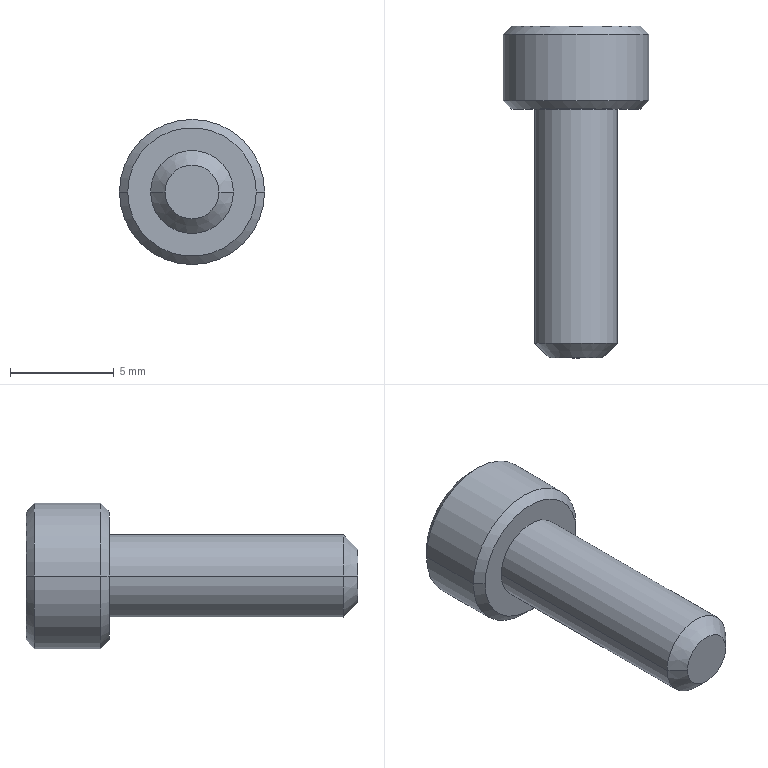Part | STEP file | BB62-M4-12L-1 | 1 solid | 27 faces | box 7 x 16 x 7 mm | volume 280.182 mm3 | plane 15 | cone 8 | cylinder 4 | commonest cylinder face diameters 4 x2 7 x2
STEP:
#1=CARTESIAN_POINT('',(0.,1.007,0.));
#2=VERTEX_POINT('',#1);
#3=CARTESIAN_POINT('',(1.72,2.,0.));
#4=VERTEX_POINT('',#3);
#5=CARTESIAN_POINT('',(0.,1.007,0.));
#6=DIRECTION('',(0.866,0.5,0.));
#7=VECTOR('',#6,1000.);
#8=LINE('',#5,#7);
#9=EDGE_CURVE('',#2,#4,#8,.T.);
#10=ORIENTED_EDGE('',*,*,#9,.F.);
#11=CARTESIAN_POINT('',(-1.72,2.,0.));
#12=VERTEX_POINT('',#11);
#13=CARTESIAN_POINT('',(0.,1.007,0.));
#14=DIRECTION('',(-0.866,0.5,0.));
#15=VECTOR('',#14,1000.);
#16=LINE('',#13,#15);
#17=EDGE_CURVE('',#2,#12,#16,.T.);
#18=ORIENTED_EDGE('',*,*,#17,.T.);
#19=CARTESIAN_POINT('',(-1.49,2.,0.86));
#20=VERTEX_POINT('',#19);
#21=CARTESIAN_POINT('',(0.,2.,0.));
#22=DIRECTION('',(0.,-1.,0.));
#23=DIRECTION('',(-1.,0.,0.));
#24=AXIS2_PLACEMENT_3D('',#21,#22,#23);
#25=CIRCLE('',#24,1.72);
#26=EDGE_CURVE('',#20,#12,#25,.T.);
#27=ORIENTED_EDGE('',*,*,#26,.F.);
#28=CARTESIAN_POINT('',(0.,2.,1.72));
#29=VERTEX_POINT('',#28);
#30=CARTESIAN_POINT('',(0.,2.,0.));
#31=DIRECTION('',(0.,-1.,0.));
#32=DIRECTION('',(-1.,0.,0.));
#33=AXIS2_PLACEMENT_3D('',#30,#31,#32);
#34=CIRCLE('',#33,1.72);
#35=EDGE_CURVE('',#29,#20,#34,.T.);
#36=ORIENTED_EDGE('',*,*,#35,.F.);
#37=CARTESIAN_POINT('',(1.49,2.,0.86));
#38=VERTEX_POINT('',#37);
#39=CARTESIAN_POINT('',(0.,2.,0.));
#40=DIRECTION('',(0.,-1.,0.));
#41=DIRECTION('',(-1.,0.,0.));
#42=AXIS2_PLACEMENT_3D('',#39,#40,#41);
#43=CIRCLE('',#42,1.72);
#44=EDGE_CURVE('',#38,#29,#43,.T.);
#45=ORIENTED_EDGE('',*,*,#44,.F.);
#46=CARTESIAN_POINT('',(0.,2.,0.));
#47=DIRECTION('',(0.,-1.,0.));
#48=DIRECTION('',(-1.,0.,0.));
#49=AXIS2_PLACEMENT_3D('',#46,#47,#48);
#50=CIRCLE('',#49,1.72);
#51=EDGE_CURVE('',#4,#38,#50,.T.);
#52=ORIENTED_EDGE('',*,*,#51,.F.);
#53=EDGE_LOOP('',(#10,#18,#27,#36,#45,#52));
#54=FACE_OUTER_BOUND('',#53,.T.);
#55=CARTESIAN_POINT('',(0.,1001.007,0.));
#56=DIRECTION('',(0.,1.,0.));
#57=DIRECTION('',(1.,0.,0.));
#58=AXIS2_PLACEMENT_3D('',#55,#56,#57);
#59=CONICAL_SURFACE('',#58,1732.051,1.047);
#60=ADVANCED_FACE('',(#54),#59,.F.);
#61=CARTESIAN_POINT('',(1.3,-12.,0.));
#62=VERTEX_POINT('',#61);
#63=CARTESIAN_POINT('',(-1.3,-12.,0.));
#64=VERTEX_POINT('',#63);
#65=CARTESIAN_POINT('',(0.,-12.,0.));
#66=DIRECTION('',(0.,1.,0.));
#67=DIRECTION('',(1.,0.,0.));
#68=AXIS2_PLACEMENT_3D('',#65,#66,#67);
#69=CIRCLE('',#68,1.3);
#70=EDGE_CURVE('',#62,#64,#69,.T.);
#71=ORIENTED_EDGE('',*,*,#70,.T.);
#72=CARTESIAN_POINT('',(-2.,-11.3,0.));
#73=VERTEX_POINT('',#72);
#74=CARTESIAN_POINT('',(-1.3,-12.,0.));
#75=DIRECTION('',(-0.7071,0.7071,0.));
#76=VECTOR('',#75,1000.);
#77=LINE('',#74,#76);
#78=EDGE_CURVE('',#64,#73,#77,.T.);
#79=ORIENTED_EDGE('',*,*,#78,.T.);
#80=CARTESIAN_POINT('',(2.,-11.3,0.));
#81=VERTEX_POINT('',#80);
#82=CARTESIAN_POINT('',(0.,-11.3,0.));
#83=DIRECTION('',(0.,-1.,0.));
#84=DIRECTION('',(-1.,0.,0.));
#85=AXIS2_PLACEMENT_3D('',#82,#83,#84);
#86=CIRCLE('',#85,2.);
#87=EDGE_CURVE('',#73,#81,#86,.T.);
#88=ORIENTED_EDGE('',*,*,#87,.T.);
#89=CARTESIAN_POINT('',(1.3,-12.,0.));
#90=DIRECTION('',(0.7071,0.7071,0.));
#91=VECTOR('',#90,1000.);
#92=LINE('',#89,#91);
#93=EDGE_CURVE('',#62,#81,#92,.T.);
#94=ORIENTED_EDGE('',*,*,#93,.F.);
#95=EDGE_LOOP('',(#71,#79,#88,#94));
#96=FACE_OUTER_BOUND('',#95,.T.);
#97=CARTESIAN_POINT('',(0.,-12.,0.));
#98=DIRECTION('',(0.,1.,0.));
#99=DIRECTION('',(1.,0.,0.));
#100=AXIS2_PLACEMENT_3D('',#97,#98,#99);
#101=CONICAL_SURFACE('',#100,1.3,0.7854);
#102=ADVANCED_FACE('',(#96),#101,.T.);
#103=ORIENTED_EDGE('',*,*,#87,.F.);
#104=CARTESIAN_POINT('',(-2.,0.,0.));
#105=VERTEX_POINT('',#104);
#106=CARTESIAN_POINT('',(-2.,-11.3,0.));
#107=DIRECTION('',(0.,1.,0.));
#108=VECTOR('',#107,1000.);
#109=LINE('',#106,#108);
#110=EDGE_CURVE('',#73,#105,#109,.T.);
#111=ORIENTED_EDGE('',*,*,#110,.T.);
#112=CARTESIAN_POINT('',(2.,0.,0.));
#113=VERTEX_POINT('',#112);
#114=CARTESIAN_POINT('',(0.,0.,0.));
#115=DIRECTION('',(0.,-1.,0.));
#116=DIRECTION('',(-1.,0.,0.));
#117=AXIS2_PLACEMENT_3D('',#114,#115,#116);
#118=CIRCLE('',#117,2.);
#119=EDGE_CURVE('',#105,#113,#118,.T.);
#120=ORIENTED_EDGE('',*,*,#119,.T.);
#121=CARTESIAN_POINT('',(2.,-11.3,0.));
#122=DIRECTION('',(0.,1.,0.));
#123=VECTOR('',#122,1000.);
#124=LINE('',#121,#123);
#125=EDGE_CURVE('',#81,#113,#124,.T.);
#126=ORIENTED_EDGE('',*,*,#125,.F.);
#127=EDGE_LOOP('',(#103,#111,#120,#126));
#128=FACE_OUTER_BOUND('',#127,.T.);
#129=CARTESIAN_POINT('',(0.,-11.3,0.));
#130=DIRECTION('',(0.,1.,0.));
#131=DIRECTION('',(1.,0.,0.));
#132=AXIS2_PLACEMENT_3D('',#129,#130,#131);
#133=CYLINDRICAL_SURFACE('',#132,2.);
#134=ADVANCED_FACE('',(#128),#133,.T.);
#135=CARTESIAN_POINT('',(-3.1,4.,0.));
#136=VERTEX_POINT('',#135);
#137=CARTESIAN_POINT('',(3.1,4.,0.));
#138=VERTEX_POINT('',#137);
#139=CARTESIAN_POINT('',(0.,4.,0.));
#140=DIRECTION('',(0.,-1.,0.));
#141=DIRECTION('',(-1.,0.,0.));
#142=AXIS2_PLACEMENT_3D('',#139,#140,#141);
#143=CIRCLE('',#142,3.1);
#144=EDGE_CURVE('',#136,#138,#143,.T.);
#145=ORIENTED_EDGE('',*,*,#144,.T.);
#146=CARTESIAN_POINT('',(3.5,3.6,0.));
#147=VERTEX_POINT('',#146);
#148=CARTESIAN_POINT('',(3.5,3.6,0.));
#149=DIRECTION('',(0.7071,-0.7071,0.));
#150=VECTOR('',#149,1000.);
#151=LINE('',#148,#150);
#152=EDGE_CURVE('',#138,#147,#151,.T.);
#153=ORIENTED_EDGE('',*,*,#152,.T.);
#154=CARTESIAN_POINT('',(-3.5,3.6,0.));
#155=VERTEX_POINT('',#154);
#156=CARTESIAN_POINT('',(0.,3.6,0.));
#157=DIRECTION('',(0.,-1.,0.));
#158=DIRECTION('',(-1.,0.,0.));
#159=AXIS2_PLACEMENT_3D('',#156,#157,#158);
#160=CIRCLE('',#159,3.5);
#161=EDGE_CURVE('',#155,#147,#160,.T.);
#162=ORIENTED_EDGE('',*,*,#161,.F.);
#163=CARTESIAN_POINT('',(-3.5,3.6,0.));
#164=DIRECTION('',(-0.7071,-0.7071,0.));
#165=VECTOR('',#164,1000.);
#166=LINE('',#163,#165);
#167=EDGE_CURVE('',#136,#155,#166,.T.);
#168=ORIENTED_EDGE('',*,*,#167,.F.);
#169=EDGE_LOOP('',(#145,#153,#162,#168));
#170=FACE_OUTER_BOUND('',#169,.T.);
#171=CARTESIAN_POINT('',(0.,3.6,0.));
#172=DIRECTION('',(0.,-1.,0.));
#173=DIRECTION('',(-1.,0.,0.));
#174=AXIS2_PLACEMENT_3D('',#171,#172,#173);
#175=CONICAL_SURFACE('',#174,3.5,0.7854);
#176=ADVANCED_FACE('',(#170),#175,.T.);
#177=ORIENTED_EDGE('',*,*,#161,.T.);
#178=CARTESIAN_POINT('',(3.5,0.4,0.));
#179=VERTEX_POINT('',#178);
#180=CARTESIAN_POINT('',(3.5,1.62,0.));
#181=DIRECTION('',(0.,-1.,0.));
#182=VECTOR('',#181,1000.);
#183=LINE('',#180,#182);
#184=EDGE_CURVE('',#147,#179,#183,.T.);
#185=ORIENTED_EDGE('',*,*,#184,.T.);
#186=CARTESIAN_POINT('',(-3.5,0.4,0.));
#187=VERTEX_POINT('',#186);
#188=CARTESIAN_POINT('',(0.,0.4,0.));
#189=DIRECTION('',(0.,-1.,0.));
#190=DIRECTION('',(-1.,0.,0.));
#191=AXIS2_PLACEMENT_3D('',#188,#189,#190);
#192=CIRCLE('',#191,3.5);
#193=EDGE_CURVE('',#187,#179,#192,.T.);
#194=ORIENTED_EDGE('',*,*,#193,.F.);
#195=CARTESIAN_POINT('',(-3.5,1.62,0.));
#196=DIRECTION('',(0.,-1.,0.));
#197=VECTOR('',#196,1000.);
#198=LINE('',#195,#197);
#199=EDGE_CURVE('',#155,#187,#198,.T.);
#200=ORIENTED_EDGE('',*,*,#199,.F.);
#201=EDGE_LOOP('',(#177,#185,#194,#200));
#202=FACE_OUTER_BOUND('',#201,.T.);
#203=CARTESIAN_POINT('',(0.,1.62,0.));
#204=DIRECTION('',(0.,-1.,0.));
#205=DIRECTION('',(-1.,0.,0.));
#206=AXIS2_PLACEMENT_3D('',#203,#204,#205);
#207=CYLINDRICAL_SURFACE('',#206,3.5);
#208=ADVANCED_FACE('',(#202),#207,.T.);
#209=CARTESIAN_POINT('',(-3.1,0.,0.));
#210=VERTEX_POINT('',#209);
#211=CARTESIAN_POINT('',(3.1,0.,0.));
#212=VERTEX_POINT('',#211);
#213=CARTESIAN_POINT('',(0.,0.,0.));
#214=DIRECTION('',(0.,-1.,0.));
#215=DIRECTION('',(-1.,0.,0.));
#216=AXIS2_PLACEMENT_3D('',#213,#214,#215);
#217=CIRCLE('',#216,3.1);
#218=EDGE_CURVE('',#210,#212,#217,.T.);
#219=ORIENTED_EDGE('',*,*,#218,.F.);
#220=CARTESIAN_POINT('',(-3.1,0.,0.));
#221=DIRECTION('',(-0.7071,0.7071,0.));
#222=VECTOR('',#221,1000.);
#223=LINE('',#220,#222);
#224=EDGE_CURVE('',#210,#187,#223,.T.);
#225=ORIENTED_EDGE('',*,*,#224,.T.);
#226=ORIENTED_EDGE('',*,*,#193,.T.);
#227=CARTESIAN_POINT('',(3.1,0.,0.));
#228=DIRECTION('',(0.7071,0.7071,0.));
#229=VECTOR('',#228,1000.);
#230=LINE('',#227,#229);
#231=EDGE_CURVE('',#212,#179,#230,.T.);
#232=ORIENTED_EDGE('',*,*,#231,.F.);
#233=EDGE_LOOP('',(#219,#225,#226,#232));
#234=FACE_OUTER_BOUND('',#233,.T.);
#235=CARTESIAN_POINT('',(0.,0.,0.));
#236=DIRECTION('',(0.,1.,0.));
#237=DIRECTION('',(1.,0.,0.));
#238=AXIS2_PLACEMENT_3D('',#235,#236,#237);
#239=CONICAL_SURFACE('',#238,3.1,0.7854);
#240=ADVANCED_FACE('',(#234),#239,.T.);
#241=ORIENTED_EDGE('',*,*,#144,.F.);
#242=CARTESIAN_POINT('',(0.,4.,0.));
#243=DIRECTION('',(0.,-1.,0.));
#244=DIRECTION('',(-1.,0.,0.));
#245=AXIS2_PLACEMENT_3D('',#242,#243,#244);
#246=CIRCLE('',#245,3.1);
#247=EDGE_CURVE('',#138,#136,#246,.T.);
#248=ORIENTED_EDGE('',*,*,#247,.F.);
#249=EDGE_LOOP('',(#241,#248));
#250=FACE_OUTER_BOUND('',#249,.T.);
#251=CARTESIAN_POINT('',(0.,4.,-1.72));
#252=VERTEX_POINT('',#251);
#253=CARTESIAN_POINT('',(-1.49,4.,-0.86));
#254=VERTEX_POINT('',#253);
#255=CARTESIAN_POINT('',(0.,4.,-1.72));
#256=DIRECTION('',(-0.866,0.,0.5));
#257=VECTOR('',#256,1000.);
#258=LINE('',#255,#257);
#259=EDGE_CURVE('',#252,#254,#258,.T.);
#260=ORIENTED_EDGE('',*,*,#259,.F.);
#261=CARTESIAN_POINT('',(1.49,4.,-0.86));
#262=VERTEX_POINT('',#261);
#263=CARTESIAN_POINT('',(1.49,4.,-0.86));
#264=DIRECTION('',(-0.866,0.,-0.5));
#265=VECTOR('',#264,1000.);
#266=LINE('',#263,#265);
#267=EDGE_CURVE('',#262,#252,#266,.T.);
#268=ORIENTED_EDGE('',*,*,#267,.F.);
#269=CARTESIAN_POINT('',(1.49,4.,0.86));
#270=VERTEX_POINT('',#269);
#271=CARTESIAN_POINT('',(1.49,4.,0.86));
#272=DIRECTION('',(0.,0.,-1.));
#273=VECTOR('',#272,1000.);
#274=LINE('',#271,#273);
#275=EDGE_CURVE('',#270,#262,#274,.T.);
#276=ORIENTED_EDGE('',*,*,#275,.F.);
#277=CARTESIAN_POINT('',(0.,4.,1.72));
#278=VERTEX_POINT('',#277);
#279=CARTESIAN_POINT('',(0.,4.,1.72));
#280=DIRECTION('',(0.866,0.,-0.5));
#281=VECTOR('',#280,1000.);
#282=LINE('',#279,#281);
#283=EDGE_CURVE('',#278,#270,#282,.T.);
#284=ORIENTED_EDGE('',*,*,#283,.F.);
#285=CARTESIAN_POINT('',(-1.49,4.,0.86));
#286=VERTEX_POINT('',#285);
#287=CARTESIAN_POINT('',(-1.49,4.,0.86));
#288=DIRECTION('',(0.866,0.,0.5));
#289=VECTOR('',#288,1000.);
#290=LINE('',#287,#289);
#291=EDGE_CURVE('',#286,#278,#290,.T.);
#292=ORIENTED_EDGE('',*,*,#291,.F.);
#293=CARTESIAN_POINT('',(-1.49,4.,-0.86));
#294=DIRECTION('',(0.,0.,1.));
#295=VECTOR('',#294,1000.);
#296=LINE('',#293,#295);
#297=EDGE_CURVE('',#254,#286,#296,.T.);
#298=ORIENTED_EDGE('',*,*,#297,.F.);
#299=EDGE_LOOP('',(#260,#268,#276,#284,#292,#298));
#300=FACE_BOUND('',#299,.T.);
#301=CARTESIAN_POINT('',(3.1,4.,0.));
#302=DIRECTION('',(0.,1.,0.));
#303=DIRECTION('',(1.,0.,0.));
#304=AXIS2_PLACEMENT_3D('',#301,#302,#303);
#305=PLANE('',#304);
#306=ADVANCED_FACE('',(#250,#300),#305,.T.);
#307=CARTESIAN_POINT('',(0.,0.,0.));
#308=DIRECTION('',(0.,-1.,0.));
#309=DIRECTION('',(-1.,0.,0.));
#310=AXIS2_PLACEMENT_3D('',#307,#308,#309);
#311=CIRCLE('',#310,2.);
#312=EDGE_CURVE('',#113,#105,#311,.T.);
#313=ORIENTED_EDGE('',*,*,#312,.F.);
#314=ORIENTED_EDGE('',*,*,#119,.F.);
#315=EDGE_LOOP('',(#313,#314));
#316=FACE_BOUND('',#315,.T.);
#317=CARTESIAN_POINT('',(0.,0.,0.));
#318=DIRECTION('',(0.,-1.,0.));
#319=DIRECTION('',(-1.,0.,0.));
#320=AXIS2_PLACEMENT_3D('',#317,#318,#319);
#321=CIRCLE('',#320,3.1);
#322=EDGE_CURVE('',#212,#210,#321,.T.);
#323=ORIENTED_EDGE('',*,*,#322,.T.);
#324=ORIENTED_EDGE('',*,*,#218,.T.);
#325=EDGE_LOOP('',(#323,#324));
#326=FACE_OUTER_BOUND('',#325,.T.);
#327=CARTESIAN_POINT('',(0.,0.,0.));
#328=DIRECTION('',(0.,-1.,0.));
#329=DIRECTION('',(-1.,0.,0.));
#330=AXIS2_PLACEMENT_3D('',#327,#328,#329);
#331=PLANE('',#330);
#332=ADVANCED_FACE('',(#316,#326),#331,.T.);
#333=ORIENTED_EDGE('',*,*,#224,.F.);
#334=ORIENTED_EDGE('',*,*,#322,.F.);
#335=ORIENTED_EDGE('',*,*,#231,.T.);
#336=CARTESIAN_POINT('',(0.,0.4,0.));
#337=DIRECTION('',(0.,-1.,0.));
#338=DIRECTION('',(-1.,0.,0.));
#339=AXIS2_PLACEMENT_3D('',#336,#337,#338);
#340=CIRCLE('',#339,3.5);
#341=EDGE_CURVE('',#179,#187,#340,.T.);
#342=ORIENTED_EDGE('',*,*,#341,.T.);
#343=EDGE_LOOP('',(#333,#334,#335,#342));
#344=FACE_OUTER_BOUND('',#343,.T.);
#345=CARTESIAN_POINT('',(0.,0.,0.));
#346=DIRECTION('',(0.,1.,0.));
#347=DIRECTION('',(1.,0.,0.));
#348=AXIS2_PLACEMENT_3D('',#345,#346,#347);
#349=CONICAL_SURFACE('',#348,3.1,0.7854);
#350=ADVANCED_FACE('',(#344),#349,.T.);
#351=ORIENTED_EDGE('',*,*,#184,.F.);
#352=CARTESIAN_POINT('',(0.,3.6,0.));
#353=DIRECTION('',(0.,-1.,0.));
#354=DIRECTION('',(-1.,0.,0.));
#355=AXIS2_PLACEMENT_3D('',#352,#353,#354);
#356=CIRCLE('',#355,3.5);
#357=EDGE_CURVE('',#147,#155,#356,.T.);
#358=ORIENTED_EDGE('',*,*,#357,.T.);
#359=ORIENTED_EDGE('',*,*,#199,.T.);
#360=ORIENTED_EDGE('',*,*,#341,.F.);
#361=EDGE_LOOP('',(#351,#358,#359,#360));
#362=FACE_OUTER_BOUND('',#361,.T.);
#363=CARTESIAN_POINT('',(0.,1.62,0.));
#364=DIRECTION('',(0.,-1.,0.));
#365=DIRECTION('',(-1.,0.,0.));
#366=AXIS2_PLACEMENT_3D('',#363,#364,#365);
#367=CYLINDRICAL_SURFACE('',#366,3.5);
#368=ADVANCED_FACE('',(#362),#367,.T.);
#369=ORIENTED_EDGE('',*,*,#152,.F.);
#370=ORIENTED_EDGE('',*,*,#247,.T.);
#371=ORIENTED_EDGE('',*,*,#167,.T.);
#372=ORIENTED_EDGE('',*,*,#357,.F.);
#373=EDGE_LOOP('',(#369,#370,#371,#372));
#374=FACE_OUTER_BOUND('',#373,.T.);
#375=CARTESIAN_POINT('',(0.,3.6,0.));
#376=DIRECTION('',(0.,-1.,0.));
#377=DIRECTION('',(-1.,0.,0.));
#378=AXIS2_PLACEMENT_3D('',#375,#376,#377);
#379=CONICAL_SURFACE('',#378,3.5,0.7854);
#380=ADVANCED_FACE('',(#374),#379,.T.);
#381=ORIENTED_EDGE('',*,*,#110,.F.);
#382=CARTESIAN_POINT('',(0.,-11.3,0.));
#383=DIRECTION('',(0.,-1.,0.));
#384=DIRECTION('',(-1.,0.,0.));
#385=AXIS2_PLACEMENT_3D('',#382,#383,#384);
#386=CIRCLE('',#385,2.);
#387=EDGE_CURVE('',#81,#73,#386,.T.);
#388=ORIENTED_EDGE('',*,*,#387,.F.);
#389=ORIENTED_EDGE('',*,*,#125,.T.);
#390=ORIENTED_EDGE('',*,*,#312,.T.);
#391=EDGE_LOOP('',(#381,#388,#389,#390));
#392=FACE_OUTER_BOUND('',#391,.T.);
#393=CARTESIAN_POINT('',(0.,-11.3,0.));
#394=DIRECTION('',(0.,1.,0.));
#395=DIRECTION('',(1.,0.,0.));
#396=AXIS2_PLACEMENT_3D('',#393,#394,#395);
#397=CYLINDRICAL_SURFACE('',#396,2.);
#398=ADVANCED_FACE('',(#392),#397,.T.);
#399=ORIENTED_EDGE('',*,*,#70,.F.);
#400=CARTESIAN_POINT('',(0.,-12.,0.));
#401=DIRECTION('',(0.,1.,0.));
#402=DIRECTION('',(1.,0.,0.));
#403=AXIS2_PLACEMENT_3D('',#400,#401,#402);
#404=CIRCLE('',#403,1.3);
#405=EDGE_CURVE('',#64,#62,#404,.T.);
#406=ORIENTED_EDGE('',*,*,#405,.F.);
#407=EDGE_LOOP('',(#399,#406));
#408=FACE_OUTER_BOUND('',#407,.T.);
#409=CARTESIAN_POINT('',(0.,-12.,0.));
#410=DIRECTION('',(0.,-1.,0.));
#411=DIRECTION('',(-1.,0.,0.));
#412=AXIS2_PLACEMENT_3D('',#409,#410,#411);
#413=PLANE('',#412);
#414=ADVANCED_FACE('',(#408),#413,.T.);
#415=ORIENTED_EDGE('',*,*,#78,.F.);
#416=ORIENTED_EDGE('',*,*,#405,.T.);
#417=ORIENTED_EDGE('',*,*,#93,.T.);
#418=ORIENTED_EDGE('',*,*,#387,.T.);
#419=EDGE_LOOP('',(#415,#416,#417,#418));
#420=FACE_OUTER_BOUND('',#419,.T.);
#421=CARTESIAN_POINT('',(0.,-12.,0.));
#422=DIRECTION('',(0.,1.,0.));
#423=DIRECTION('',(1.,0.,0.));
#424=AXIS2_PLACEMENT_3D('',#421,#422,#423);
#425=CONICAL_SURFACE('',#424,1.3,0.7854);
#426=ADVANCED_FACE('',(#420),#425,.T.);
#427=CARTESIAN_POINT('',(1.49,2.,-0.86));
#428=VERTEX_POINT('',#427);
#429=CARTESIAN_POINT('',(0.,2.,-1.72));
#430=VERTEX_POINT('',#429);
#431=CARTESIAN_POINT('',(1.49,2.,-0.86));
#432=DIRECTION('',(-0.866,0.,-0.5));
#433=VECTOR('',#432,1000.);
#434=LINE('',#431,#433);
#435=EDGE_CURVE('',#428,#430,#434,.T.);
#436=ORIENTED_EDGE('',*,*,#435,.F.);
#437=CARTESIAN_POINT('',(1.49,4.,-0.86));
#438=DIRECTION('',(0.,-1.,0.));
#439=VECTOR('',#438,1000.);
#440=LINE('',#437,#439);
#441=EDGE_CURVE('',#262,#428,#440,.T.);
#442=ORIENTED_EDGE('',*,*,#441,.F.);
#443=ORIENTED_EDGE('',*,*,#267,.T.);
#444=CARTESIAN_POINT('',(0.,4.,-1.72));
#445=DIRECTION('',(0.,-1.,0.));
#446=VECTOR('',#445,1000.);
#447=LINE('',#444,#446);
#448=EDGE_CURVE('',#252,#430,#447,.T.);
#449=ORIENTED_EDGE('',*,*,#448,.T.);
#450=EDGE_LOOP('',(#436,#442,#443,#449));
#451=FACE_OUTER_BOUND('',#450,.T.);
#452=CARTESIAN_POINT('',(1.49,4.,-0.86));
#453=DIRECTION('',(-0.5,0.,0.866));
#454=DIRECTION('',(0.866,0.,0.5));
#455=AXIS2_PLACEMENT_3D('',#452,#453,#454);
#456=PLANE('',#455);
#457=ADVANCED_FACE('',(#451),#456,.T.);
#458=CARTESIAN_POINT('',(-1.49,2.,-0.86));
#459=VERTEX_POINT('',#458);
#460=CARTESIAN_POINT('',(0.,2.,-1.72));
#461=DIRECTION('',(-0.866,0.,0.5));
#462=VECTOR('',#461,1000.);
#463=LINE('',#460,#462);
#464=EDGE_CURVE('',#430,#459,#463,.T.);
#465=ORIENTED_EDGE('',*,*,#464,.F.);
#466=ORIENTED_EDGE('',*,*,#448,.F.);
#467=ORIENTED_EDGE('',*,*,#259,.T.);
#468=CARTESIAN_POINT('',(-1.49,4.,-0.86));
#469=DIRECTION('',(0.,-1.,0.));
#470=VECTOR('',#469,1000.);
#471=LINE('',#468,#470);
#472=EDGE_CURVE('',#254,#459,#471,.T.);
#473=ORIENTED_EDGE('',*,*,#472,.T.);
#474=EDGE_LOOP('',(#465,#466,#467,#473));
#475=FACE_OUTER_BOUND('',#474,.T.);
#476=CARTESIAN_POINT('',(0.,4.,-1.72));
#477=DIRECTION('',(0.5,0.,0.866));
#478=DIRECTION('',(0.866,0.,-0.5));
#479=AXIS2_PLACEMENT_3D('',#476,#477,#478);
#480=PLANE('',#479);
#481=ADVANCED_FACE('',(#475),#480,.T.);
#482=CARTESIAN_POINT('',(-1.49,2.,-0.86));
#483=DIRECTION('',(0.,0.,1.));
#484=VECTOR('',#483,1000.);
#485=LINE('',#482,#484);
#486=EDGE_CURVE('',#459,#20,#485,.T.);
#487=ORIENTED_EDGE('',*,*,#486,.F.);
#488=ORIENTED_EDGE('',*,*,#472,.F.);
#489=ORIENTED_EDGE('',*,*,#297,.T.);
#490=CARTESIAN_POINT('',(-1.49,4.,0.86));
#491=DIRECTION('',(0.,-1.,0.));
#492=VECTOR('',#491,1000.);
#493=LINE('',#490,#492);
#494=EDGE_CURVE('',#286,#20,#493,.T.);
#495=ORIENTED_EDGE('',*,*,#494,.T.);
#496=EDGE_LOOP('',(#487,#488,#489,#495));
#497=FACE_OUTER_BOUND('',#496,.T.);
#498=CARTESIAN_POINT('',(-1.49,4.,-0.86));
#499=DIRECTION('',(1.,0.,0.));
#500=DIRECTION('',(0.,0.,-1.));
#501=AXIS2_PLACEMENT_3D('',#498,#499,#500);
#502=PLANE('',#501);
#503=ADVANCED_FACE('',(#497),#502,.T.);
#504=CARTESIAN_POINT('',(-1.49,2.,0.86));
#505=DIRECTION('',(0.866,0.,0.5));
#506=VECTOR('',#505,1000.);
#507=LINE('',#504,#506);
#508=EDGE_CURVE('',#20,#29,#507,.T.);
#509=ORIENTED_EDGE('',*,*,#508,.F.);
#510=ORIENTED_EDGE('',*,*,#494,.F.);
#511=ORIENTED_EDGE('',*,*,#291,.T.);
#512=CARTESIAN_POINT('',(0.,4.,1.72));
#513=DIRECTION('',(0.,-1.,0.));
#514=VECTOR('',#513,1000.);
#515=LINE('',#512,#514);
#516=EDGE_CURVE('',#278,#29,#515,.T.);
#517=ORIENTED_EDGE('',*,*,#516,.T.);
#518=EDGE_LOOP('',(#509,#510,#511,#517));
#519=FACE_OUTER_BOUND('',#518,.T.);
#520=CARTESIAN_POINT('',(-1.49,4.,0.86));
#521=DIRECTION('',(0.5,0.,-0.866));
#522=DIRECTION('',(-0.866,0.,-0.5));
#523=AXIS2_PLACEMENT_3D('',#520,#521,#522);
#524=PLANE('',#523);
#525=ADVANCED_FACE('',(#519),#524,.T.);
#526=CARTESIAN_POINT('',(0.,2.,1.72));
#527=DIRECTION('',(0.866,0.,-0.5));
#528=VECTOR('',#527,1000.);
#529=LINE('',#526,#528);
#530=EDGE_CURVE('',#29,#38,#529,.T.);
#531=ORIENTED_EDGE('',*,*,#530,.F.);
#532=ORIENTED_EDGE('',*,*,#516,.F.);
#533=ORIENTED_EDGE('',*,*,#283,.T.);
#534=CARTESIAN_POINT('',(1.49,4.,0.86));
#535=DIRECTION('',(0.,-1.,0.));
#536=VECTOR('',#535,1000.);
#537=LINE('',#534,#536);
#538=EDGE_CURVE('',#270,#38,#537,.T.);
#539=ORIENTED_EDGE('',*,*,#538,.T.);
#540=EDGE_LOOP('',(#531,#532,#533,#539));
#541=FACE_OUTER_BOUND('',#540,.T.);
#542=CARTESIAN_POINT('',(0.,4.,1.72));
#543=DIRECTION('',(-0.5,0.,-0.866));
#544=DIRECTION('',(-0.866,0.,0.5));
#545=AXIS2_PLACEMENT_3D('',#542,#543,#544);
#546=PLANE('',#545);
#547=ADVANCED_FACE('',(#541),#546,.T.);
#548=CARTESIAN_POINT('',(1.49,2.,0.86));
#549=DIRECTION('',(0.,0.,-1.));
#550=VECTOR('',#549,1000.);
#551=LINE('',#548,#550);
#552=EDGE_CURVE('',#38,#428,#551,.T.);
#553=ORIENTED_EDGE('',*,*,#552,.F.);
#554=ORIENTED_EDGE('',*,*,#538,.F.);
#555=ORIENTED_EDGE('',*,*,#275,.T.);
#556=ORIENTED_EDGE('',*,*,#441,.T.);
#557=EDGE_LOOP('',(#553,#554,#555,#556));
#558=FACE_OUTER_BOUND('',#557,.T.);
#559=CARTESIAN_POINT('',(1.49,4.,0.86));
#560=DIRECTION('',(-1.,0.,0.));
#561=DIRECTION('',(0.,0.,1.));
#562=AXIS2_PLACEMENT_3D('',#559,#560,#561);
#563=PLANE('',#562);
#564=ADVANCED_FACE('',(#558),#563,.T.);
#565=ORIENTED_EDGE('',*,*,#435,.T.);
#566=CARTESIAN_POINT('',(0.,2.,0.));
#567=DIRECTION('',(0.,-1.,0.));
#568=DIRECTION('',(-1.,0.,0.));
#569=AXIS2_PLACEMENT_3D('',#566,#567,#568);
#570=CIRCLE('',#569,1.72);
#571=EDGE_CURVE('',#430,#428,#570,.T.);
#572=ORIENTED_EDGE('',*,*,#571,.T.);
#573=EDGE_LOOP('',(#565,#572));
#574=FACE_OUTER_BOUND('',#573,.T.);
#575=CARTESIAN_POINT('',(0.,2.,0.));
#576=DIRECTION('',(0.,1.,0.));
#577=DIRECTION('',(1.,0.,0.));
#578=AXIS2_PLACEMENT_3D('',#575,#576,#577);
#579=PLANE('',#578);
#580=ADVANCED_FACE('',(#574),#579,.F.);
#581=ORIENTED_EDGE('',*,*,#552,.T.);
#582=CARTESIAN_POINT('',(0.,2.,0.));
#583=DIRECTION('',(0.,-1.,0.));
#584=DIRECTION('',(-1.,0.,0.));
#585=AXIS2_PLACEMENT_3D('',#582,#583,#584);
#586=CIRCLE('',#585,1.72);
#587=EDGE_CURVE('',#428,#4,#586,.T.);
#588=ORIENTED_EDGE('',*,*,#587,.T.);
#589=ORIENTED_EDGE('',*,*,#51,.T.);
#590=EDGE_LOOP('',(#581,#588,#589));
#591=FACE_OUTER_BOUND('',#590,.T.);
#592=CARTESIAN_POINT('',(0.,2.,0.));
#593=DIRECTION('',(0.,1.,0.));
#594=DIRECTION('',(1.,0.,0.));
#595=AXIS2_PLACEMENT_3D('',#592,#593,#594);
#596=PLANE('',#595);
#597=ADVANCED_FACE('',(#591),#596,.F.);
#598=ORIENTED_EDGE('',*,*,#530,.T.);
#599=ORIENTED_EDGE('',*,*,#44,.T.);
#600=EDGE_LOOP('',(#598,#599));
#601=FACE_OUTER_BOUND('',#600,.T.);
#602=CARTESIAN_POINT('',(0.,2.,0.));
#603=DIRECTION('',(0.,1.,0.));
#604=DIRECTION('',(1.,0.,0.));
#605=AXIS2_PLACEMENT_3D('',#602,#603,#604);
#606=PLANE('',#605);
#607=ADVANCED_FACE('',(#601),#606,.F.);
#608=ORIENTED_EDGE('',*,*,#508,.T.);
#609=ORIENTED_EDGE('',*,*,#35,.T.);
#610=EDGE_LOOP('',(#608,#609));
#611=FACE_OUTER_BOUND('',#610,.T.);
#612=CARTESIAN_POINT('',(0.,2.,0.));
#613=DIRECTION('',(0.,1.,0.));
#614=DIRECTION('',(1.,0.,0.));
#615=AXIS2_PLACEMENT_3D('',#612,#613,#614);
#616=PLANE('',#615);
#617=ADVANCED_FACE('',(#611),#616,.F.);
#618=ORIENTED_EDGE('',*,*,#486,.T.);
#619=ORIENTED_EDGE('',*,*,#26,.T.);
#620=CARTESIAN_POINT('',(0.,2.,0.));
#621=DIRECTION('',(0.,-1.,0.));
#622=DIRECTION('',(-1.,0.,0.));
#623=AXIS2_PLACEMENT_3D('',#620,#621,#622);
#624=CIRCLE('',#623,1.72);
#625=EDGE_CURVE('',#12,#459,#624,.T.);
#626=ORIENTED_EDGE('',*,*,#625,.T.);
#627=EDGE_LOOP('',(#618,#619,#626));
#628=FACE_OUTER_BOUND('',#627,.T.);
#629=CARTESIAN_POINT('',(0.,2.,0.));
#630=DIRECTION('',(0.,1.,0.));
#631=DIRECTION('',(1.,0.,0.));
#632=AXIS2_PLACEMENT_3D('',#629,#630,#631);
#633=PLANE('',#632);
#634=ADVANCED_FACE('',(#628),#633,.F.);
#635=ORIENTED_EDGE('',*,*,#464,.T.);
#636=CARTESIAN_POINT('',(0.,2.,0.));
#637=DIRECTION('',(0.,-1.,0.));
#638=DIRECTION('',(-1.,0.,0.));
#639=AXIS2_PLACEMENT_3D('',#636,#637,#638);
#640=CIRCLE('',#639,1.72);
#641=EDGE_CURVE('',#459,#430,#640,.T.);
#642=ORIENTED_EDGE('',*,*,#641,.T.);
#643=EDGE_LOOP('',(#635,#642));
#644=FACE_OUTER_BOUND('',#643,.T.);
#645=CARTESIAN_POINT('',(0.,2.,0.));
#646=DIRECTION('',(0.,1.,0.));
#647=DIRECTION('',(1.,0.,0.));
#648=AXIS2_PLACEMENT_3D('',#645,#646,#647);
#649=PLANE('',#648);
#650=ADVANCED_FACE('',(#644),#649,.F.);
#651=ORIENTED_EDGE('',*,*,#17,.F.);
#652=ORIENTED_EDGE('',*,*,#9,.T.);
#653=ORIENTED_EDGE('',*,*,#587,.F.);
#654=ORIENTED_EDGE('',*,*,#571,.F.);
#655=ORIENTED_EDGE('',*,*,#641,.F.);
#656=ORIENTED_EDGE('',*,*,#625,.F.);
#657=EDGE_LOOP('',(#651,#652,#653,#654,#655,#656));
#658=FACE_OUTER_BOUND('',#657,.T.);
#659=CARTESIAN_POINT('',(0.,1001.007,0.));
#660=DIRECTION('',(0.,1.,0.));
#661=DIRECTION('',(1.,0.,0.));
#662=AXIS2_PLACEMENT_3D('',#659,#660,#661);
#663=CONICAL_SURFACE('',#662,1732.051,1.047);
#664=ADVANCED_FACE('',(#658),#663,.F.);
#665=CLOSED_SHELL('',(#60,#102,#134,#176,#208,#240,#306,#332,#350,#368,#380,#398,#414,#426,#457,#481,#503,#525,#547,#564,#580,#597,#607,#617,#634,#650,#664));
#666=MANIFOLD_SOLID_BREP('',#665);
#667=CARTESIAN_POINT('',(0.,0.,0.));
#668=DIRECTION('',(0.,0.,1.));
#669=DIRECTION('',(1.,0.,0.));
#670=AXIS2_PLACEMENT_3D('',#667,#668,#669);
#671=(LENGTH_UNIT()NAMED_UNIT(*)SI_UNIT(.MILLI.,.METRE.));
#672=UNCERTAINTY_MEASURE_WITH_UNIT(LENGTH_MEASURE(0.00001),#671,'','');
#673=(NAMED_UNIT(*)PLANE_ANGLE_UNIT()SI_UNIT($,.RADIAN.));
#674=(NAMED_UNIT(*)SI_UNIT($,.STERADIAN.)SOLID_ANGLE_UNIT());
#675=(GEOMETRIC_REPRESENTATION_CONTEXT(3)GLOBAL_UNCERTAINTY_ASSIGNED_CONTEXT((#672))GLOBAL_UNIT_ASSIGNED_CONTEXT((#671,#673,#674))REPRESENTATION_CONTEXT('',''));
#676=ADVANCED_BREP_SHAPE_REPRESENTATION('',(#666,#670),#675);